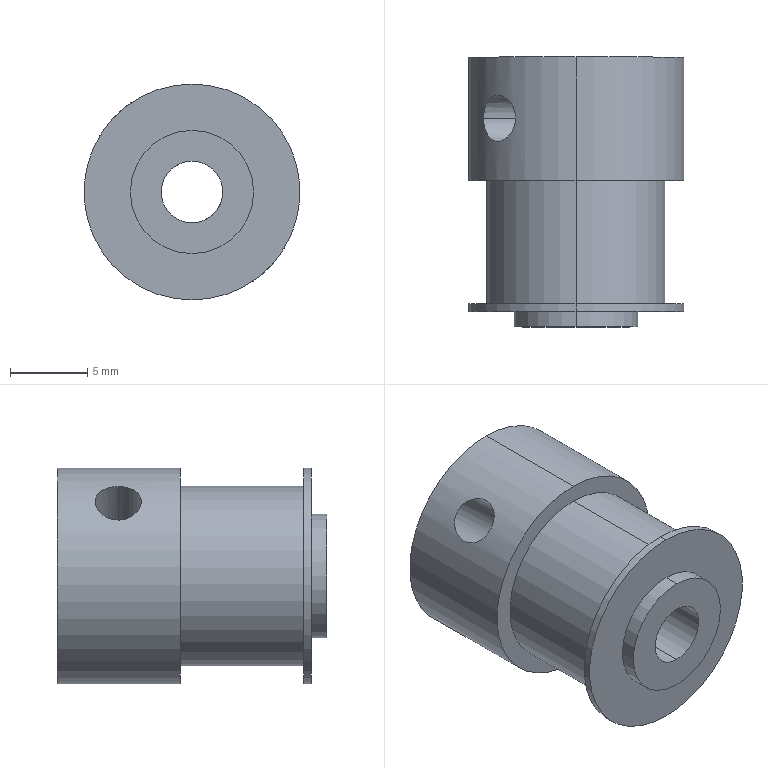Part | SolidWorks | features BaseBody 1 | 1 solid | 19 faces | box 14 x 17.5 x 14 mm | volume 1918 mm3 | cylinder 14 | plane 5 | commonest cylinder face diameters 3 x4 14 x4 4 x2 8 x2 11.64 x2
STEP:
#1=CARTESIAN_POINT('',(-3.92,13.536,5.799));
#2=VERTEX_POINT('',#1);
#3=CARTESIAN_POINT('',(-5.988,13.536,3.626));
#4=VERTEX_POINT('',#3);
#5=CARTESIAN_POINT('',(-3.92,13.536,5.799));
#6=CARTESIAN_POINT('',(-3.92,13.34,5.799));
#7=CARTESIAN_POINT('',(-3.954,13.142,5.777));
#8=CARTESIAN_POINT('',(-4.079,12.781,5.689));
#9=CARTESIAN_POINT('',(-4.171,12.615,5.623));
#10=CARTESIAN_POINT('',(-4.337,12.407,5.495));
#11=CARTESIAN_POINT('',(-4.398,12.344,5.446));
#12=CARTESIAN_POINT('',(-4.524,12.235,5.342));
#13=CARTESIAN_POINT('',(-4.59,12.189,5.286));
#14=CARTESIAN_POINT('',(-4.794,12.076,5.104));
#15=CARTESIAN_POINT('',(-4.935,12.036,4.968));
#16=CARTESIAN_POINT('',(-5.14,12.036,4.753));
#17=CARTESIAN_POINT('',(-5.205,12.046,4.681));
#18=CARTESIAN_POINT('',(-5.332,12.084,4.536));
#19=CARTESIAN_POINT('',(-5.394,12.113,4.463));
#20=CARTESIAN_POINT('',(-5.565,12.226,4.25));
#21=CARTESIAN_POINT('',(-5.664,12.337,4.115));
#22=CARTESIAN_POINT('',(-5.824,12.613,3.886));
#23=CARTESIAN_POINT('',(-5.885,12.779,3.791));
#24=CARTESIAN_POINT('',(-5.967,13.14,3.661));
#25=CARTESIAN_POINT('',(-5.988,13.337,3.626));
#26=CARTESIAN_POINT('',(-5.988,13.536,3.626));
#27=B_SPLINE_CURVE_WITH_KNOTS('',3,(#5,#6,#7,#8,#9,#10,#11,#12,#13,#14,#15,#16,#17,#18,#19,#20,#21,#22,#23,#24,#25,#26),.UNSPECIFIED.,.F.,.F.,(4,2,2,2,2,2,2,2,2,2,4),(0.004703,0.005291,0.005879,0.006173,0.006467,0.007054,0.007348,0.007642,0.00823,0.008818,0.009405),.UNSPECIFIED.);
#28=EDGE_CURVE('',#2,#4,#27,.T.);
#29=ORIENTED_EDGE('',*,*,#28,.F.);
#30=CARTESIAN_POINT('',(0.07529,13.536,1.999));
#31=VERTEX_POINT('',#30);
#32=CARTESIAN_POINT('',(6.106,13.536,-3.738));
#33=DIRECTION('',(0.7246,0.,-0.6892));
#34=VECTOR('',#33,1000.);
#35=LINE('',#32,#34);
#36=EDGE_CURVE('',#2,#31,#35,.T.);
#37=ORIENTED_EDGE('',*,*,#36,.T.);
#38=CARTESIAN_POINT('',(0.,13.149,2.));
#39=VERTEX_POINT('',#38);
#40=CARTESIAN_POINT('',(0.07529,13.536,1.999));
#41=CARTESIAN_POINT('',(0.07529,13.47,1.999));
#42=CARTESIAN_POINT('',(0.06851,13.404,1.999));
#43=CARTESIAN_POINT('',(0.04292,13.274,2.));
#44=CARTESIAN_POINT('',(0.02403,13.211,2.));
#45=CARTESIAN_POINT('',(0.,13.149,2.));
#46=B_SPLINE_CURVE_WITH_KNOTS('',3,(#40,#41,#42,#43,#44,#45),.UNSPECIFIED.,.F.,.F.,(4,2,4),(0.004899,0.005095,0.005291),.UNSPECIFIED.);
#47=EDGE_CURVE('',#31,#39,#46,.T.);
#48=ORIENTED_EDGE('',*,*,#47,.T.);
#49=CARTESIAN_POINT('',(-1.992,13.536,-0.1751));
#50=VERTEX_POINT('',#49);
#51=CARTESIAN_POINT('',(0.,13.149,2.));
#52=CARTESIAN_POINT('',(-0.06898,12.971,2.));
#53=CARTESIAN_POINT('',(-0.1759,12.813,1.996));
#54=CARTESIAN_POINT('',(-0.4253,12.53,1.958));
#55=CARTESIAN_POINT('',(-0.569,12.406,1.924));
#56=CARTESIAN_POINT('',(-0.7916,12.256,1.838));
#57=CARTESIAN_POINT('',(-0.8669,12.212,1.804));
#58=CARTESIAN_POINT('',(-1.019,12.136,1.723));
#59=CARTESIAN_POINT('',(-1.096,12.105,1.675));
#60=CARTESIAN_POINT('',(-1.32,12.036,1.514));
#61=CARTESIAN_POINT('',(-1.46,12.025,1.379));
#62=CARTESIAN_POINT('',(-1.633,12.061,1.158));
#63=CARTESIAN_POINT('',(-1.686,12.082,1.08));
#64=CARTESIAN_POINT('',(-1.776,12.14,0.9237));
#65=CARTESIAN_POINT('',(-1.815,12.176,0.8447));
#66=CARTESIAN_POINT('',(-1.913,12.306,0.6092));
#67=CARTESIAN_POINT('',(-1.952,12.417,0.4576));
#68=CARTESIAN_POINT('',(-1.996,12.677,0.1855));
#69=CARTESIAN_POINT('',(-2.001,12.826,0.06354));
#70=CARTESIAN_POINT('',(-1.999,13.158,-0.1174));
#71=CARTESIAN_POINT('',(-1.992,13.345,-0.1751));
#72=CARTESIAN_POINT('',(-1.992,13.536,-0.1751));
#73=B_SPLINE_CURVE_WITH_KNOTS('',3,(#51,#52,#53,#54,#55,#56,#57,#58,#59,#60,#61,#62,#63,#64,#65,#66,#67,#68,#69,#70,#71,#72),.UNSPECIFIED.,.F.,.F.,(4,2,2,2,2,2,2,2,2,2,4),(0.005291,0.005853,0.006416,0.006697,0.006978,0.00754,0.007821,0.008102,0.008665,0.009227,0.009789),.UNSPECIFIED.);
#74=EDGE_CURVE('',#39,#50,#73,.T.);
#75=ORIENTED_EDGE('',*,*,#74,.T.);
#76=CARTESIAN_POINT('',(4.038,13.536,-5.911));
#77=DIRECTION('',(0.7246,0.,-0.6892));
#78=VECTOR('',#77,1000.);
#79=LINE('',#76,#78);
#80=EDGE_CURVE('',#4,#50,#79,.T.);
#81=ORIENTED_EDGE('',*,*,#80,.F.);
#82=EDGE_LOOP('',(#29,#37,#48,#75,#81));
#83=FACE_OUTER_BOUND('',#82,.T.);
#84=CARTESIAN_POINT('',(5.072,13.536,-4.824));
#85=DIRECTION('',(0.7246,0.,-0.6892));
#86=DIRECTION('',(-0.6892,0.,-0.7246));
#87=AXIS2_PLACEMENT_3D('',#84,#85,#86);
#88=CYLINDRICAL_SURFACE('',#87,1.5);
#89=ADVANCED_FACE('',(#83),#88,.F.);
#90=CARTESIAN_POINT('',(0.,13.149,-2.));
#91=VERTEX_POINT('',#90);
#92=CARTESIAN_POINT('',(1.992,13.536,0.1751));
#93=VERTEX_POINT('',#92);
#94=CARTESIAN_POINT('',(0.,13.149,-2.));
#95=CARTESIAN_POINT('',(0.06867,12.972,-2.));
#96=CARTESIAN_POINT('',(0.1764,12.812,-1.996));
#97=CARTESIAN_POINT('',(0.4248,12.531,-1.958));
#98=CARTESIAN_POINT('',(0.5678,12.407,-1.924));
#99=CARTESIAN_POINT('',(0.7916,12.256,-1.838));
#100=CARTESIAN_POINT('',(0.8673,12.212,-1.804));
#101=CARTESIAN_POINT('',(1.02,12.136,-1.722));
#102=CARTESIAN_POINT('',(1.098,12.104,-1.674));
#103=CARTESIAN_POINT('',(1.246,12.059,-1.567));
#104=CARTESIAN_POINT('',(1.319,12.044,-1.506));
#105=CARTESIAN_POINT('',(1.456,12.033,-1.375));
#106=CARTESIAN_POINT('',(1.519,12.037,-1.305));
#107=CARTESIAN_POINT('',(1.692,12.073,-1.083));
#108=CARTESIAN_POINT('',(1.783,12.134,-0.9215));
#109=CARTESIAN_POINT('',(1.913,12.306,-0.6088));
#110=CARTESIAN_POINT('',(1.952,12.418,-0.4567));
#111=CARTESIAN_POINT('',(1.996,12.677,-0.1853));
#112=CARTESIAN_POINT('',(2.001,12.827,-0.063));
#113=CARTESIAN_POINT('',(1.999,13.158,0.1174));
#114=CARTESIAN_POINT('',(1.992,13.344,0.1751));
#115=CARTESIAN_POINT('',(1.992,13.536,0.1751));
#116=B_SPLINE_CURVE_WITH_KNOTS('',3,(#94,#95,#96,#97,#98,#99,#100,#101,#102,#103,#104,#105,#106,#107,#108,#109,#110,#111,#112,#113,#114,#115),.UNSPECIFIED.,.F.,.F.,(4,2,2,2,2,2,2,2,2,2,4),(0.0007898,0.001356,0.001923,0.002206,0.00249,0.002773,0.003056,0.003623,0.004189,0.004756,0.005323),.UNSPECIFIED.);
#117=EDGE_CURVE('',#91,#93,#116,.T.);
#118=ORIENTED_EDGE('',*,*,#117,.T.);
#119=CARTESIAN_POINT('',(5.988,13.536,-3.626));
#120=VERTEX_POINT('',#119);
#121=CARTESIAN_POINT('',(6.106,13.536,-3.738));
#122=DIRECTION('',(0.7246,0.,-0.6892));
#123=VECTOR('',#122,1000.);
#124=LINE('',#121,#123);
#125=EDGE_CURVE('',#93,#120,#124,.T.);
#126=ORIENTED_EDGE('',*,*,#125,.T.);
#127=CARTESIAN_POINT('',(3.92,13.536,-5.799));
#128=VERTEX_POINT('',#127);
#129=CARTESIAN_POINT('',(3.92,13.536,-5.799));
#130=CARTESIAN_POINT('',(3.92,13.437,-5.799));
#131=CARTESIAN_POINT('',(3.929,13.339,-5.794));
#132=CARTESIAN_POINT('',(3.961,13.147,-5.772));
#133=CARTESIAN_POINT('',(3.985,13.052,-5.755));
#134=CARTESIAN_POINT('',(4.048,12.87,-5.711));
#135=CARTESIAN_POINT('',(4.087,12.784,-5.683));
#136=CARTESIAN_POINT('',(4.176,12.621,-5.618));
#137=CARTESIAN_POINT('',(4.227,12.544,-5.58));
#138=CARTESIAN_POINT('',(4.393,12.337,-5.452));
#139=CARTESIAN_POINT('',(4.523,12.226,-5.345));
#140=CARTESIAN_POINT('',(4.794,12.076,-5.104));
#141=CARTESIAN_POINT('',(4.936,12.036,-4.967));
#142=CARTESIAN_POINT('',(5.139,12.036,-4.754));
#143=CARTESIAN_POINT('',(5.206,12.046,-4.68));
#144=CARTESIAN_POINT('',(5.333,12.085,-4.535));
#145=CARTESIAN_POINT('',(5.394,12.113,-4.463));
#146=CARTESIAN_POINT('',(5.565,12.226,-4.25));
#147=CARTESIAN_POINT('',(5.664,12.336,-4.116));
#148=CARTESIAN_POINT('',(5.785,12.545,-3.942));
#149=CARTESIAN_POINT('',(5.82,12.621,-3.89));
#150=CARTESIAN_POINT('',(5.88,12.783,-3.798));
#151=CARTESIAN_POINT('',(5.906,12.871,-3.758));
#152=CARTESIAN_POINT('',(5.947,13.052,-3.693));
#153=CARTESIAN_POINT('',(5.962,13.146,-3.668));
#154=CARTESIAN_POINT('',(5.983,13.339,-3.634));
#155=CARTESIAN_POINT('',(5.988,13.438,-3.626));
#156=CARTESIAN_POINT('',(5.988,13.536,-3.626));
#157=B_SPLINE_CURVE_WITH_KNOTS('',3,(#129,#130,#131,#132,#133,#134,#135,#136,#137,#138,#139,#140,#141,#142,#143,#144,#145,#146,#147,#148,#149,#150,#151,#152,#153,#154,#155,#156),.UNSPECIFIED.,.F.,.F.,(4,2,2,2,2,2,2,2,2,2,2,2,2,4),(0.,0.000294,0.0005879,0.0008819,0.001176,0.001764,0.002352,0.002646,0.00294,0.003527,0.003821,0.004115,0.004409,0.004703),.UNSPECIFIED.);
#158=EDGE_CURVE('',#128,#120,#157,.T.);
#159=ORIENTED_EDGE('',*,*,#158,.F.);
#160=CARTESIAN_POINT('',(-0.07529,13.536,-1.999));
#161=VERTEX_POINT('',#160);
#162=CARTESIAN_POINT('',(4.038,13.536,-5.911));
#163=DIRECTION('',(0.7246,0.,-0.6892));
#164=VECTOR('',#163,1000.);
#165=LINE('',#162,#164);
#166=EDGE_CURVE('',#161,#128,#165,.T.);
#167=ORIENTED_EDGE('',*,*,#166,.F.);
#168=CARTESIAN_POINT('',(-0.07529,13.536,-1.999));
#169=CARTESIAN_POINT('',(-0.07529,13.47,-1.999));
#170=CARTESIAN_POINT('',(-0.06861,13.404,-1.999));
#171=CARTESIAN_POINT('',(-0.04307,13.275,-2.));
#172=CARTESIAN_POINT('',(-0.02394,13.211,-2.));
#173=CARTESIAN_POINT('',(0.,13.149,-2.));
#174=B_SPLINE_CURVE_WITH_KNOTS('',3,(#168,#169,#170,#171,#172,#173),.UNSPECIFIED.,.F.,.F.,(4,2,4),(0.0003947,0.0005923,0.0007898),.UNSPECIFIED.);
#175=EDGE_CURVE('',#161,#91,#174,.T.);
#176=ORIENTED_EDGE('',*,*,#175,.T.);
#177=EDGE_LOOP('',(#118,#126,#159,#167,#176));
#178=FACE_OUTER_BOUND('',#177,.T.);
#179=CARTESIAN_POINT('',(5.072,13.536,-4.824));
#180=DIRECTION('',(0.7246,0.,-0.6892));
#181=DIRECTION('',(-0.6892,0.,-0.7246));
#182=AXIS2_PLACEMENT_3D('',#179,#180,#181);
#183=CYLINDRICAL_SURFACE('',#182,1.5);
#184=ADVANCED_FACE('',(#178),#183,.F.);
#185=ORIENTED_EDGE('',*,*,#158,.T.);
#186=CARTESIAN_POINT('',(5.988,13.536,-3.626));
#187=CARTESIAN_POINT('',(5.988,13.732,-3.626));
#188=CARTESIAN_POINT('',(5.967,13.93,-3.66));
#189=CARTESIAN_POINT('',(5.886,14.291,-3.79));
#190=CARTESIAN_POINT('',(5.825,14.458,-3.885));
#191=CARTESIAN_POINT('',(5.705,14.665,-4.057));
#192=CARTESIAN_POINT('',(5.66,14.729,-4.12));
#193=CARTESIAN_POINT('',(5.562,14.837,-4.251));
#194=CARTESIAN_POINT('',(5.509,14.883,-4.32));
#195=CARTESIAN_POINT('',(5.337,14.997,-4.533));
#196=CARTESIAN_POINT('',(5.209,15.036,-4.68));
#197=CARTESIAN_POINT('',(5.004,15.036,-4.896));
#198=CARTESIAN_POINT('',(4.935,15.027,-4.965));
#199=CARTESIAN_POINT('',(4.797,14.988,-5.099));
#200=CARTESIAN_POINT('',(4.727,14.959,-5.164));
#201=CARTESIAN_POINT('',(4.523,14.847,-5.345));
#202=CARTESIAN_POINT('',(4.393,14.735,-5.452));
#203=CARTESIAN_POINT('',(4.173,14.46,-5.622));
#204=CARTESIAN_POINT('',(4.08,14.293,-5.689));
#205=CARTESIAN_POINT('',(3.955,13.932,-5.776));
#206=CARTESIAN_POINT('',(3.92,13.735,-5.799));
#207=CARTESIAN_POINT('',(3.92,13.536,-5.799));
#208=B_SPLINE_CURVE_WITH_KNOTS('',3,(#186,#187,#188,#189,#190,#191,#192,#193,#194,#195,#196,#197,#198,#199,#200,#201,#202,#203,#204,#205,#206,#207),.UNSPECIFIED.,.F.,.F.,(4,2,2,2,2,2,2,2,2,2,4),(0.004703,0.005291,0.005879,0.006173,0.006467,0.007054,0.007348,0.007642,0.00823,0.008818,0.009405),.UNSPECIFIED.);
#209=EDGE_CURVE('',#120,#128,#208,.T.);
#210=ORIENTED_EDGE('',*,*,#209,.T.);
#211=EDGE_LOOP('',(#185,#210));
#212=FACE_BOUND('',#211,.T.);
#213=CARTESIAN_POINT('',(0.,17.5,7.));
#214=VERTEX_POINT('',#213);
#215=CARTESIAN_POINT('',(0.,17.5,-7.));
#216=VERTEX_POINT('',#215);
#217=CARTESIAN_POINT('',(0.,17.5,0.));
#218=DIRECTION('',(0.,1.,0.));
#219=DIRECTION('',(0.,0.,1.));
#220=AXIS2_PLACEMENT_3D('',#217,#218,#219);
#221=CIRCLE('',#220,7.);
#222=EDGE_CURVE('',#214,#216,#221,.T.);
#223=ORIENTED_EDGE('',*,*,#222,.F.);
#224=CARTESIAN_POINT('',(0.,9.5,7.));
#225=VERTEX_POINT('',#224);
#226=CARTESIAN_POINT('',(0.,17.5,7.));
#227=DIRECTION('',(0.,-1.,0.));
#228=VECTOR('',#227,1000.);
#229=LINE('',#226,#228);
#230=EDGE_CURVE('',#214,#225,#229,.T.);
#231=ORIENTED_EDGE('',*,*,#230,.T.);
#232=CARTESIAN_POINT('',(0.,9.5,-7.));
#233=VERTEX_POINT('',#232);
#234=CARTESIAN_POINT('',(0.,9.5,0.));
#235=DIRECTION('',(0.,1.,0.));
#236=DIRECTION('',(0.,0.,1.));
#237=AXIS2_PLACEMENT_3D('',#234,#235,#236);
#238=CIRCLE('',#237,7.);
#239=EDGE_CURVE('',#225,#233,#238,.T.);
#240=ORIENTED_EDGE('',*,*,#239,.T.);
#241=CARTESIAN_POINT('',(0.,17.5,-7.));
#242=DIRECTION('',(0.,-1.,0.));
#243=VECTOR('',#242,1000.);
#244=LINE('',#241,#243);
#245=EDGE_CURVE('',#216,#233,#244,.T.);
#246=ORIENTED_EDGE('',*,*,#245,.F.);
#247=EDGE_LOOP('',(#223,#231,#240,#246));
#248=FACE_OUTER_BOUND('',#247,.T.);
#249=CARTESIAN_POINT('',(0.,17.5,0.));
#250=DIRECTION('',(0.,-1.,0.));
#251=DIRECTION('',(0.,0.,-1.));
#252=AXIS2_PLACEMENT_3D('',#249,#250,#251);
#253=CYLINDRICAL_SURFACE('',#252,7.);
#254=ADVANCED_FACE('',(#212,#248),#253,.T.);
#255=CARTESIAN_POINT('',(0.,9.5,5.82));
#256=VERTEX_POINT('',#255);
#257=CARTESIAN_POINT('',(0.,9.5,-5.82));
#258=VERTEX_POINT('',#257);
#259=CARTESIAN_POINT('',(0.,9.5,0.));
#260=DIRECTION('',(0.,1.,0.));
#261=DIRECTION('',(0.,0.,1.));
#262=AXIS2_PLACEMENT_3D('',#259,#260,#261);
#263=CIRCLE('',#262,5.82);
#264=EDGE_CURVE('',#256,#258,#263,.T.);
#265=ORIENTED_EDGE('',*,*,#264,.F.);
#266=CARTESIAN_POINT('',(0.,1.5,5.82));
#267=VERTEX_POINT('',#266);
#268=CARTESIAN_POINT('',(0.,9.5,5.82));
#269=DIRECTION('',(0.,-1.,0.));
#270=VECTOR('',#269,1000.);
#271=LINE('',#268,#270);
#272=EDGE_CURVE('',#256,#267,#271,.T.);
#273=ORIENTED_EDGE('',*,*,#272,.T.);
#274=CARTESIAN_POINT('',(0.,1.5,-5.82));
#275=VERTEX_POINT('',#274);
#276=CARTESIAN_POINT('',(0.,1.5,0.));
#277=DIRECTION('',(0.,1.,0.));
#278=DIRECTION('',(0.,0.,1.));
#279=AXIS2_PLACEMENT_3D('',#276,#277,#278);
#280=CIRCLE('',#279,5.82);
#281=EDGE_CURVE('',#267,#275,#280,.T.);
#282=ORIENTED_EDGE('',*,*,#281,.T.);
#283=CARTESIAN_POINT('',(0.,9.5,-5.82));
#284=DIRECTION('',(0.,-1.,0.));
#285=VECTOR('',#284,1000.);
#286=LINE('',#283,#285);
#287=EDGE_CURVE('',#258,#275,#286,.T.);
#288=ORIENTED_EDGE('',*,*,#287,.F.);
#289=EDGE_LOOP('',(#265,#273,#282,#288));
#290=FACE_OUTER_BOUND('',#289,.T.);
#291=CARTESIAN_POINT('',(0.,9.5,0.));
#292=DIRECTION('',(0.,-1.,0.));
#293=DIRECTION('',(0.,0.,-1.));
#294=AXIS2_PLACEMENT_3D('',#291,#292,#293);
#295=CYLINDRICAL_SURFACE('',#294,5.82);
#296=ADVANCED_FACE('',(#290),#295,.T.);
#297=CARTESIAN_POINT('',(0.,1.5,7.));
#298=VERTEX_POINT('',#297);
#299=CARTESIAN_POINT('',(0.,1.5,-7.));
#300=VERTEX_POINT('',#299);
#301=CARTESIAN_POINT('',(0.,1.5,0.));
#302=DIRECTION('',(0.,1.,0.));
#303=DIRECTION('',(0.,0.,1.));
#304=AXIS2_PLACEMENT_3D('',#301,#302,#303);
#305=CIRCLE('',#304,7.);
#306=EDGE_CURVE('',#298,#300,#305,.T.);
#307=ORIENTED_EDGE('',*,*,#306,.F.);
#308=CARTESIAN_POINT('',(0.,1.,7.));
#309=VERTEX_POINT('',#308);
#310=CARTESIAN_POINT('',(0.,1.5,7.));
#311=DIRECTION('',(0.,-1.,0.));
#312=VECTOR('',#311,1000.);
#313=LINE('',#310,#312);
#314=EDGE_CURVE('',#298,#309,#313,.T.);
#315=ORIENTED_EDGE('',*,*,#314,.T.);
#316=CARTESIAN_POINT('',(0.,1.,-7.));
#317=VERTEX_POINT('',#316);
#318=CARTESIAN_POINT('',(0.,1.,0.));
#319=DIRECTION('',(0.,1.,0.));
#320=DIRECTION('',(0.,0.,1.));
#321=AXIS2_PLACEMENT_3D('',#318,#319,#320);
#322=CIRCLE('',#321,7.);
#323=EDGE_CURVE('',#309,#317,#322,.T.);
#324=ORIENTED_EDGE('',*,*,#323,.T.);
#325=CARTESIAN_POINT('',(0.,1.5,-7.));
#326=DIRECTION('',(0.,-1.,0.));
#327=VECTOR('',#326,1000.);
#328=LINE('',#325,#327);
#329=EDGE_CURVE('',#300,#317,#328,.T.);
#330=ORIENTED_EDGE('',*,*,#329,.F.);
#331=EDGE_LOOP('',(#307,#315,#324,#330));
#332=FACE_OUTER_BOUND('',#331,.T.);
#333=CARTESIAN_POINT('',(0.,1.5,0.));
#334=DIRECTION('',(0.,-1.,0.));
#335=DIRECTION('',(0.,0.,-1.));
#336=AXIS2_PLACEMENT_3D('',#333,#334,#335);
#337=CYLINDRICAL_SURFACE('',#336,7.);
#338=ADVANCED_FACE('',(#332),#337,.T.);
#339=CARTESIAN_POINT('',(0.,17.5,-2.));
#340=VERTEX_POINT('',#339);
#341=CARTESIAN_POINT('',(0.,17.5,2.));
#342=VERTEX_POINT('',#341);
#343=CARTESIAN_POINT('',(0.,17.5,0.));
#344=DIRECTION('',(0.,1.,0.));
#345=DIRECTION('',(0.,0.,1.));
#346=AXIS2_PLACEMENT_3D('',#343,#344,#345);
#347=CIRCLE('',#346,2.);
#348=EDGE_CURVE('',#340,#342,#347,.T.);
#349=ORIENTED_EDGE('',*,*,#348,.T.);
#350=CARTESIAN_POINT('',(0.,13.924,2.));
#351=VERTEX_POINT('',#350);
#352=CARTESIAN_POINT('',(0.,1.,2.));
#353=DIRECTION('',(0.,-1.,0.));
#354=VECTOR('',#353,1000.);
#355=LINE('',#352,#354);
#356=EDGE_CURVE('',#342,#351,#355,.T.);
#357=ORIENTED_EDGE('',*,*,#356,.T.);
#358=CARTESIAN_POINT('',(-1.992,13.536,-0.1751));
#359=CARTESIAN_POINT('',(-1.992,13.632,-0.1751));
#360=CARTESIAN_POINT('',(-1.994,13.725,-0.1613));
#361=CARTESIAN_POINT('',(-1.997,13.906,-0.1106));
#362=CARTESIAN_POINT('',(-1.999,13.995,-0.07313));
#363=CARTESIAN_POINT('',(-2.001,14.245,0.06217));
#364=CARTESIAN_POINT('',(-1.996,14.394,0.1841));
#365=CARTESIAN_POINT('',(-1.952,14.654,0.4554));
#366=CARTESIAN_POINT('',(-1.913,14.765,0.6074));
#367=CARTESIAN_POINT('',(-1.786,14.936,0.9159));
#368=CARTESIAN_POINT('',(-1.695,14.997,1.077));
#369=CARTESIAN_POINT('',(-1.465,15.048,1.374));
#370=CARTESIAN_POINT('',(-1.325,15.037,1.509));
#371=CARTESIAN_POINT('',(-1.026,14.947,1.727));
#372=CARTESIAN_POINT('',(-0.8688,14.868,1.809));
#373=CARTESIAN_POINT('',(-0.5697,14.667,1.924));
#374=CARTESIAN_POINT('',(-0.4258,14.543,1.958));
#375=CARTESIAN_POINT('',(-0.1768,14.261,1.996));
#376=CARTESIAN_POINT('',(-0.06869,14.101,2.));
#377=CARTESIAN_POINT('',(0.,13.924,2.));
#378=B_SPLINE_CURVE_WITH_KNOTS('',3,(#358,#359,#360,#361,#362,#363,#364,#365,#366,#367,#368,#369,#370,#371,#372,#373,#374,#375,#376,#377),.UNSPECIFIED.,.F.,.F.,(4,2,2,2,2,2,2,2,2,4),(0.,0.0002817,0.0005634,0.001127,0.00169,0.002254,0.002817,0.003381,0.003944,0.004507),.UNSPECIFIED.);
#379=EDGE_CURVE('',#50,#351,#378,.T.);
#380=ORIENTED_EDGE('',*,*,#379,.F.);
#381=ORIENTED_EDGE('',*,*,#74,.F.);
#382=CARTESIAN_POINT('',(0.,0.,2.));
#383=VERTEX_POINT('',#382);
#384=CARTESIAN_POINT('',(0.,1.,2.));
#385=DIRECTION('',(0.,-1.,0.));
#386=VECTOR('',#385,1000.);
#387=LINE('',#384,#386);
#388=EDGE_CURVE('',#39,#383,#387,.T.);
#389=ORIENTED_EDGE('',*,*,#388,.T.);
#390=CARTESIAN_POINT('',(0.,0.,-2.));
#391=VERTEX_POINT('',#390);
#392=CARTESIAN_POINT('',(0.,0.,0.));
#393=DIRECTION('',(0.,1.,0.));
#394=DIRECTION('',(0.,0.,1.));
#395=AXIS2_PLACEMENT_3D('',#392,#393,#394);
#396=CIRCLE('',#395,2.);
#397=EDGE_CURVE('',#391,#383,#396,.T.);
#398=ORIENTED_EDGE('',*,*,#397,.F.);
#399=CARTESIAN_POINT('',(0.,1.,-2.));
#400=DIRECTION('',(0.,-1.,0.));
#401=VECTOR('',#400,1000.);
#402=LINE('',#399,#401);
#403=EDGE_CURVE('',#91,#391,#402,.T.);
#404=ORIENTED_EDGE('',*,*,#403,.F.);
#405=ORIENTED_EDGE('',*,*,#175,.F.);
#406=CARTESIAN_POINT('',(0.,13.924,-2.));
#407=VERTEX_POINT('',#406);
#408=CARTESIAN_POINT('',(0.,13.924,-2.));
#409=CARTESIAN_POINT('',(-0.0241,13.861,-2.));
#410=CARTESIAN_POINT('',(-0.04289,13.798,-2.));
#411=CARTESIAN_POINT('',(-0.0685,13.669,-1.999));
#412=CARTESIAN_POINT('',(-0.07529,13.603,-1.999));
#413=CARTESIAN_POINT('',(-0.07529,13.536,-1.999));
#414=B_SPLINE_CURVE_WITH_KNOTS('',3,(#408,#409,#410,#411,#412,#413),.UNSPECIFIED.,.F.,.F.,(4,2,4),(0.,0.0001974,0.0003947),.UNSPECIFIED.);
#415=EDGE_CURVE('',#407,#161,#414,.T.);
#416=ORIENTED_EDGE('',*,*,#415,.F.);
#417=CARTESIAN_POINT('',(0.,1.,-2.));
#418=DIRECTION('',(0.,-1.,0.));
#419=VECTOR('',#418,1000.);
#420=LINE('',#417,#419);
#421=EDGE_CURVE('',#340,#407,#420,.T.);
#422=ORIENTED_EDGE('',*,*,#421,.F.);
#423=EDGE_LOOP('',(#349,#357,#380,#381,#389,#398,#404,#405,#416,#422));
#424=FACE_OUTER_BOUND('',#423,.T.);
#425=CARTESIAN_POINT('',(0.,1.,0.));
#426=DIRECTION('',(0.,-1.,0.));
#427=DIRECTION('',(0.,0.,-1.));
#428=AXIS2_PLACEMENT_3D('',#425,#426,#427);
#429=CYLINDRICAL_SURFACE('',#428,2.);
#430=ADVANCED_FACE('',(#424),#429,.F.);
#431=CARTESIAN_POINT('',(0.,1.,4.));
#432=VERTEX_POINT('',#431);
#433=CARTESIAN_POINT('',(0.,1.,-4.));
#434=VERTEX_POINT('',#433);
#435=CARTESIAN_POINT('',(0.,1.,0.));
#436=DIRECTION('',(0.,1.,0.));
#437=DIRECTION('',(0.,0.,1.));
#438=AXIS2_PLACEMENT_3D('',#435,#436,#437);
#439=CIRCLE('',#438,4.);
#440=EDGE_CURVE('',#432,#434,#439,.T.);
#441=ORIENTED_EDGE('',*,*,#440,.F.);
#442=CARTESIAN_POINT('',(0.,0.,4.));
#443=VERTEX_POINT('',#442);
#444=CARTESIAN_POINT('',(0.,1.,4.));
#445=DIRECTION('',(0.,-1.,0.));
#446=VECTOR('',#445,1000.);
#447=LINE('',#444,#446);
#448=EDGE_CURVE('',#432,#443,#447,.T.);
#449=ORIENTED_EDGE('',*,*,#448,.T.);
#450=CARTESIAN_POINT('',(0.,0.,-4.));
#451=VERTEX_POINT('',#450);
#452=CARTESIAN_POINT('',(0.,0.,0.));
#453=DIRECTION('',(0.,1.,0.));
#454=DIRECTION('',(0.,0.,1.));
#455=AXIS2_PLACEMENT_3D('',#452,#453,#454);
#456=CIRCLE('',#455,4.);
#457=EDGE_CURVE('',#443,#451,#456,.T.);
#458=ORIENTED_EDGE('',*,*,#457,.T.);
#459=CARTESIAN_POINT('',(0.,1.,-4.));
#460=DIRECTION('',(0.,-1.,0.));
#461=VECTOR('',#460,1000.);
#462=LINE('',#459,#461);
#463=EDGE_CURVE('',#434,#451,#462,.T.);
#464=ORIENTED_EDGE('',*,*,#463,.F.);
#465=EDGE_LOOP('',(#441,#449,#458,#464));
#466=FACE_OUTER_BOUND('',#465,.T.);
#467=CARTESIAN_POINT('',(0.,1.,0.));
#468=DIRECTION('',(0.,-1.,0.));
#469=DIRECTION('',(0.,0.,-1.));
#470=AXIS2_PLACEMENT_3D('',#467,#468,#469);
#471=CYLINDRICAL_SURFACE('',#470,4.);
#472=ADVANCED_FACE('',(#466),#471,.T.);
#473=CARTESIAN_POINT('',(0.,1.5,0.));
#474=DIRECTION('',(0.,1.,0.));
#475=DIRECTION('',(0.,0.,1.));
#476=AXIS2_PLACEMENT_3D('',#473,#474,#475);
#477=CIRCLE('',#476,7.);
#478=EDGE_CURVE('',#300,#298,#477,.T.);
#479=ORIENTED_EDGE('',*,*,#478,.T.);
#480=ORIENTED_EDGE('',*,*,#306,.T.);
#481=EDGE_LOOP('',(#479,#480));
#482=FACE_OUTER_BOUND('',#481,.T.);
#483=CARTESIAN_POINT('',(0.,1.5,0.));
#484=DIRECTION('',(0.,1.,0.));
#485=DIRECTION('',(0.,0.,1.));
#486=AXIS2_PLACEMENT_3D('',#483,#484,#485);
#487=CIRCLE('',#486,5.82);
#488=EDGE_CURVE('',#275,#267,#487,.T.);
#489=ORIENTED_EDGE('',*,*,#488,.F.);
#490=ORIENTED_EDGE('',*,*,#281,.F.);
#491=EDGE_LOOP('',(#489,#490));
#492=FACE_BOUND('',#491,.T.);
#493=CARTESIAN_POINT('',(0.,1.5,0.));
#494=DIRECTION('',(0.,1.,0.));
#495=DIRECTION('',(0.,0.,1.));
#496=AXIS2_PLACEMENT_3D('',#493,#494,#495);
#497=PLANE('',#496);
#498=ADVANCED_FACE('',(#482,#492),#497,.T.);
#499=CARTESIAN_POINT('',(0.,0.,0.));
#500=DIRECTION('',(0.,1.,0.));
#501=DIRECTION('',(0.,0.,1.));
#502=AXIS2_PLACEMENT_3D('',#499,#500,#501);
#503=CIRCLE('',#502,4.);
#504=EDGE_CURVE('',#451,#443,#503,.T.);
#505=ORIENTED_EDGE('',*,*,#504,.F.);
#506=ORIENTED_EDGE('',*,*,#457,.F.);
#507=EDGE_LOOP('',(#505,#506));
#508=FACE_OUTER_BOUND('',#507,.T.);
#509=ORIENTED_EDGE('',*,*,#397,.T.);
#510=CARTESIAN_POINT('',(0.,0.,0.));
#511=DIRECTION('',(0.,1.,0.));
#512=DIRECTION('',(0.,0.,1.));
#513=AXIS2_PLACEMENT_3D('',#510,#511,#512);
#514=CIRCLE('',#513,2.);
#515=EDGE_CURVE('',#383,#391,#514,.T.);
#516=ORIENTED_EDGE('',*,*,#515,.T.);
#517=EDGE_LOOP('',(#509,#516));
#518=FACE_BOUND('',#517,.T.);
#519=CARTESIAN_POINT('',(0.,0.,0.));
#520=DIRECTION('',(0.,1.,0.));
#521=DIRECTION('',(0.,0.,1.));
#522=AXIS2_PLACEMENT_3D('',#519,#520,#521);
#523=PLANE('',#522);
#524=ADVANCED_FACE('',(#508,#518),#523,.F.);
#525=ORIENTED_EDGE('',*,*,#448,.F.);
#526=CARTESIAN_POINT('',(0.,1.,0.));
#527=DIRECTION('',(0.,1.,0.));
#528=DIRECTION('',(0.,0.,1.));
#529=AXIS2_PLACEMENT_3D('',#526,#527,#528);
#530=CIRCLE('',#529,4.);
#531=EDGE_CURVE('',#434,#432,#530,.T.);
#532=ORIENTED_EDGE('',*,*,#531,.F.);
#533=ORIENTED_EDGE('',*,*,#463,.T.);
#534=ORIENTED_EDGE('',*,*,#504,.T.);
#535=EDGE_LOOP('',(#525,#532,#533,#534));
#536=FACE_OUTER_BOUND('',#535,.T.);
#537=CARTESIAN_POINT('',(0.,1.,0.));
#538=DIRECTION('',(0.,-1.,0.));
#539=DIRECTION('',(0.,0.,-1.));
#540=AXIS2_PLACEMENT_3D('',#537,#538,#539);
#541=CYLINDRICAL_SURFACE('',#540,4.);
#542=ADVANCED_FACE('',(#536),#541,.T.);
#543=ORIENTED_EDGE('',*,*,#356,.F.);
#544=CARTESIAN_POINT('',(0.,17.5,0.));
#545=DIRECTION('',(0.,1.,0.));
#546=DIRECTION('',(0.,0.,1.));
#547=AXIS2_PLACEMENT_3D('',#544,#545,#546);
#548=CIRCLE('',#547,2.);
#549=EDGE_CURVE('',#342,#340,#548,.T.);
#550=ORIENTED_EDGE('',*,*,#549,.T.);
#551=ORIENTED_EDGE('',*,*,#421,.T.);
#552=CARTESIAN_POINT('',(1.992,13.536,0.1751));
#553=CARTESIAN_POINT('',(1.992,13.728,0.1751));
#554=CARTESIAN_POINT('',(1.999,13.914,0.1175));
#555=CARTESIAN_POINT('',(2.001,14.245,-0.06258));
#556=CARTESIAN_POINT('',(1.996,14.395,-0.1848));
#557=CARTESIAN_POINT('',(1.952,14.653,-0.4548));
#558=CARTESIAN_POINT('',(1.913,14.765,-0.6073));
#559=CARTESIAN_POINT('',(1.785,14.937,-0.9174));
#560=CARTESIAN_POINT('',(1.695,14.998,-1.078));
#561=CARTESIAN_POINT('',(1.464,15.048,-1.375));
#562=CARTESIAN_POINT('',(1.324,15.037,-1.51));
#563=CARTESIAN_POINT('',(1.026,14.947,-1.727));
#564=CARTESIAN_POINT('',(0.8687,14.868,-1.809));
#565=CARTESIAN_POINT('',(0.57,14.667,-1.924));
#566=CARTESIAN_POINT('',(0.4262,14.543,-1.958));
#567=CARTESIAN_POINT('',(0.1772,14.262,-1.996));
#568=CARTESIAN_POINT('',(0.06914,14.102,-2.));
#569=CARTESIAN_POINT('',(0.,13.924,-2.));
#570=B_SPLINE_CURVE_WITH_KNOTS('',3,(#552,#553,#554,#555,#556,#557,#558,#559,#560,#561,#562,#563,#564,#565,#566,#567,#568,#569),.UNSPECIFIED.,.F.,.F.,(4,2,2,2,2,2,2,2,4),(0.005323,0.005889,0.006455,0.007021,0.007587,0.008154,0.00872,0.009286,0.009852),.UNSPECIFIED.);
#571=EDGE_CURVE('',#93,#407,#570,.T.);
#572=ORIENTED_EDGE('',*,*,#571,.F.);
#573=ORIENTED_EDGE('',*,*,#117,.F.);
#574=ORIENTED_EDGE('',*,*,#403,.T.);
#575=ORIENTED_EDGE('',*,*,#515,.F.);
#576=ORIENTED_EDGE('',*,*,#388,.F.);
#577=ORIENTED_EDGE('',*,*,#47,.F.);
#578=CARTESIAN_POINT('',(0.,13.924,2.));
#579=CARTESIAN_POINT('',(0.0239,13.862,2.));
#580=CARTESIAN_POINT('',(0.04305,13.798,2.));
#581=CARTESIAN_POINT('',(0.06862,13.668,1.999));
#582=CARTESIAN_POINT('',(0.07529,13.603,1.999));
#583=CARTESIAN_POINT('',(0.07529,13.536,1.999));
#584=B_SPLINE_CURVE_WITH_KNOTS('',3,(#578,#579,#580,#581,#582,#583),.UNSPECIFIED.,.F.,.F.,(4,2,4),(0.004507,0.004703,0.004899),.UNSPECIFIED.);
#585=EDGE_CURVE('',#351,#31,#584,.T.);
#586=ORIENTED_EDGE('',*,*,#585,.F.);
#587=EDGE_LOOP('',(#543,#550,#551,#572,#573,#574,#575,#576,#577,#586));
#588=FACE_OUTER_BOUND('',#587,.T.);
#589=CARTESIAN_POINT('',(0.,1.,0.));
#590=DIRECTION('',(0.,-1.,0.));
#591=DIRECTION('',(0.,0.,-1.));
#592=AXIS2_PLACEMENT_3D('',#589,#590,#591);
#593=CYLINDRICAL_SURFACE('',#592,2.);
#594=ADVANCED_FACE('',(#588),#593,.F.);
#595=CARTESIAN_POINT('',(0.,1.,0.));
#596=DIRECTION('',(0.,1.,0.));
#597=DIRECTION('',(0.,0.,1.));
#598=AXIS2_PLACEMENT_3D('',#595,#596,#597);
#599=CIRCLE('',#598,7.);
#600=EDGE_CURVE('',#317,#309,#599,.T.);
#601=ORIENTED_EDGE('',*,*,#600,.F.);
#602=ORIENTED_EDGE('',*,*,#323,.F.);
#603=EDGE_LOOP('',(#601,#602));
#604=FACE_OUTER_BOUND('',#603,.T.);
#605=ORIENTED_EDGE('',*,*,#531,.T.);
#606=ORIENTED_EDGE('',*,*,#440,.T.);
#607=EDGE_LOOP('',(#605,#606));
#608=FACE_BOUND('',#607,.T.);
#609=CARTESIAN_POINT('',(0.,1.,0.));
#610=DIRECTION('',(0.,1.,0.));
#611=DIRECTION('',(0.,0.,1.));
#612=AXIS2_PLACEMENT_3D('',#609,#610,#611);
#613=PLANE('',#612);
#614=ADVANCED_FACE('',(#604,#608),#613,.F.);
#615=ORIENTED_EDGE('',*,*,#314,.F.);
#616=ORIENTED_EDGE('',*,*,#478,.F.);
#617=ORIENTED_EDGE('',*,*,#329,.T.);
#618=ORIENTED_EDGE('',*,*,#600,.T.);
#619=EDGE_LOOP('',(#615,#616,#617,#618));
#620=FACE_OUTER_BOUND('',#619,.T.);
#621=CARTESIAN_POINT('',(0.,1.5,0.));
#622=DIRECTION('',(0.,-1.,0.));
#623=DIRECTION('',(0.,0.,-1.));
#624=AXIS2_PLACEMENT_3D('',#621,#622,#623);
#625=CYLINDRICAL_SURFACE('',#624,7.);
#626=ADVANCED_FACE('',(#620),#625,.T.);
#627=ORIENTED_EDGE('',*,*,#272,.F.);
#628=CARTESIAN_POINT('',(0.,9.5,0.));
#629=DIRECTION('',(0.,1.,0.));
#630=DIRECTION('',(0.,0.,1.));
#631=AXIS2_PLACEMENT_3D('',#628,#629,#630);
#632=CIRCLE('',#631,5.82);
#633=EDGE_CURVE('',#258,#256,#632,.T.);
#634=ORIENTED_EDGE('',*,*,#633,.F.);
#635=ORIENTED_EDGE('',*,*,#287,.T.);
#636=ORIENTED_EDGE('',*,*,#488,.T.);
#637=EDGE_LOOP('',(#627,#634,#635,#636));
#638=FACE_OUTER_BOUND('',#637,.T.);
#639=CARTESIAN_POINT('',(0.,9.5,0.));
#640=DIRECTION('',(0.,-1.,0.));
#641=DIRECTION('',(0.,0.,-1.));
#642=AXIS2_PLACEMENT_3D('',#639,#640,#641);
#643=CYLINDRICAL_SURFACE('',#642,5.82);
#644=ADVANCED_FACE('',(#638),#643,.T.);
#645=CARTESIAN_POINT('',(0.,9.5,0.));
#646=DIRECTION('',(0.,1.,0.));
#647=DIRECTION('',(0.,0.,1.));
#648=AXIS2_PLACEMENT_3D('',#645,#646,#647);
#649=CIRCLE('',#648,7.);
#650=EDGE_CURVE('',#233,#225,#649,.T.);
#651=ORIENTED_EDGE('',*,*,#650,.F.);
#652=ORIENTED_EDGE('',*,*,#239,.F.);
#653=EDGE_LOOP('',(#651,#652));
#654=FACE_OUTER_BOUND('',#653,.T.);
#655=ORIENTED_EDGE('',*,*,#633,.T.);
#656=ORIENTED_EDGE('',*,*,#264,.T.);
#657=EDGE_LOOP('',(#655,#656));
#658=FACE_BOUND('',#657,.T.);
#659=CARTESIAN_POINT('',(0.,9.5,0.));
#660=DIRECTION('',(0.,1.,0.));
#661=DIRECTION('',(0.,0.,1.));
#662=AXIS2_PLACEMENT_3D('',#659,#660,#661);
#663=PLANE('',#662);
#664=ADVANCED_FACE('',(#654,#658),#663,.F.);
#665=CARTESIAN_POINT('',(0.,17.5,0.));
#666=DIRECTION('',(0.,1.,0.));
#667=DIRECTION('',(0.,0.,1.));
#668=AXIS2_PLACEMENT_3D('',#665,#666,#667);
#669=CIRCLE('',#668,7.);
#670=EDGE_CURVE('',#216,#214,#669,.T.);
#671=ORIENTED_EDGE('',*,*,#670,.T.);
#672=ORIENTED_EDGE('',*,*,#222,.T.);
#673=EDGE_LOOP('',(#671,#672));
#674=FACE_OUTER_BOUND('',#673,.T.);
#675=ORIENTED_EDGE('',*,*,#348,.F.);
#676=ORIENTED_EDGE('',*,*,#549,.F.);
#677=EDGE_LOOP('',(#675,#676));
#678=FACE_BOUND('',#677,.T.);
#679=CARTESIAN_POINT('',(0.,17.5,0.));
#680=DIRECTION('',(0.,1.,0.));
#681=DIRECTION('',(0.,0.,1.));
#682=AXIS2_PLACEMENT_3D('',#679,#680,#681);
#683=PLANE('',#682);
#684=ADVANCED_FACE('',(#674,#678),#683,.T.);
#685=ORIENTED_EDGE('',*,*,#230,.F.);
#686=ORIENTED_EDGE('',*,*,#670,.F.);
#687=ORIENTED_EDGE('',*,*,#245,.T.);
#688=ORIENTED_EDGE('',*,*,#650,.T.);
#689=EDGE_LOOP('',(#685,#686,#687,#688));
#690=FACE_OUTER_BOUND('',#689,.T.);
#691=CARTESIAN_POINT('',(-5.988,13.536,3.626));
#692=CARTESIAN_POINT('',(-5.988,13.636,3.626));
#693=CARTESIAN_POINT('',(-5.983,13.733,3.634));
#694=CARTESIAN_POINT('',(-5.962,13.926,3.667));
#695=CARTESIAN_POINT('',(-5.947,14.021,3.693));
#696=CARTESIAN_POINT('',(-5.906,14.202,3.758));
#697=CARTESIAN_POINT('',(-5.881,14.288,3.797));
#698=CARTESIAN_POINT('',(-5.82,14.451,3.89));
#699=CARTESIAN_POINT('',(-5.784,14.528,3.943));
#700=CARTESIAN_POINT('',(-5.665,14.735,4.115));
#701=CARTESIAN_POINT('',(-5.565,14.847,4.25));
#702=CARTESIAN_POINT('',(-5.338,14.997,4.532));
#703=CARTESIAN_POINT('',(-5.208,15.036,4.682));
#704=CARTESIAN_POINT('',(-5.005,15.036,4.895));
#705=CARTESIAN_POINT('',(-4.934,15.026,4.966));
#706=CARTESIAN_POINT('',(-4.796,14.988,5.1));
#707=CARTESIAN_POINT('',(-4.727,14.96,5.164));
#708=CARTESIAN_POINT('',(-4.523,14.846,5.346));
#709=CARTESIAN_POINT('',(-4.394,14.736,5.451));
#710=CARTESIAN_POINT('',(-4.227,14.527,5.58));
#711=CARTESIAN_POINT('',(-4.176,14.452,5.618));
#712=CARTESIAN_POINT('',(-4.087,14.289,5.683));
#713=CARTESIAN_POINT('',(-4.048,14.202,5.711));
#714=CARTESIAN_POINT('',(-3.985,14.02,5.755));
#715=CARTESIAN_POINT('',(-3.961,13.927,5.771));
#716=CARTESIAN_POINT('',(-3.929,13.734,5.794));
#717=CARTESIAN_POINT('',(-3.92,13.634,5.799));
#718=CARTESIAN_POINT('',(-3.92,13.536,5.799));
#719=B_SPLINE_CURVE_WITH_KNOTS('',3,(#691,#692,#693,#694,#695,#696,#697,#698,#699,#700,#701,#702,#703,#704,#705,#706,#707,#708,#709,#710,#711,#712,#713,#714,#715,#716,#717,#718),.UNSPECIFIED.,.F.,.F.,(4,2,2,2,2,2,2,2,2,2,2,2,2,4),(0.,0.000294,0.0005879,0.0008819,0.001176,0.001764,0.002352,0.002646,0.00294,0.003527,0.003821,0.004115,0.004409,0.004703),.UNSPECIFIED.);
#720=EDGE_CURVE('',#4,#2,#719,.T.);
#721=ORIENTED_EDGE('',*,*,#720,.T.);
#722=ORIENTED_EDGE('',*,*,#28,.T.);
#723=EDGE_LOOP('',(#721,#722));
#724=FACE_BOUND('',#723,.T.);
#725=CARTESIAN_POINT('',(0.,17.5,0.));
#726=DIRECTION('',(0.,-1.,0.));
#727=DIRECTION('',(0.,0.,-1.));
#728=AXIS2_PLACEMENT_3D('',#725,#726,#727);
#729=CYLINDRICAL_SURFACE('',#728,7.);
#730=ADVANCED_FACE('',(#690,#724),#729,.T.);
#731=ORIENTED_EDGE('',*,*,#125,.F.);
#732=ORIENTED_EDGE('',*,*,#571,.T.);
#733=ORIENTED_EDGE('',*,*,#415,.T.);
#734=ORIENTED_EDGE('',*,*,#166,.T.);
#735=ORIENTED_EDGE('',*,*,#209,.F.);
#736=EDGE_LOOP('',(#731,#732,#733,#734,#735));
#737=FACE_OUTER_BOUND('',#736,.T.);
#738=CARTESIAN_POINT('',(5.072,13.536,-4.824));
#739=DIRECTION('',(0.7246,0.,-0.6892));
#740=DIRECTION('',(-0.6892,0.,-0.7246));
#741=AXIS2_PLACEMENT_3D('',#738,#739,#740);
#742=CYLINDRICAL_SURFACE('',#741,1.5);
#743=ADVANCED_FACE('',(#737),#742,.F.);
#744=ORIENTED_EDGE('',*,*,#36,.F.);
#745=ORIENTED_EDGE('',*,*,#720,.F.);
#746=ORIENTED_EDGE('',*,*,#80,.T.);
#747=ORIENTED_EDGE('',*,*,#379,.T.);
#748=ORIENTED_EDGE('',*,*,#585,.T.);
#749=EDGE_LOOP('',(#744,#745,#746,#747,#748));
#750=FACE_OUTER_BOUND('',#749,.T.);
#751=CARTESIAN_POINT('',(5.072,13.536,-4.824));
#752=DIRECTION('',(0.7246,0.,-0.6892));
#753=DIRECTION('',(-0.6892,0.,-0.7246));
#754=AXIS2_PLACEMENT_3D('',#751,#752,#753);
#755=CYLINDRICAL_SURFACE('',#754,1.5);
#756=ADVANCED_FACE('',(#750),#755,.F.);
#757=CLOSED_SHELL('',(#89,#184,#254,#296,#338,#430,#472,#498,#524,#542,#594,#614,#626,#644,#664,#684,#730,#743,#756));
#758=MANIFOLD_SOLID_BREP('',#757);
#759=CARTESIAN_POINT('',(0.,0.,0.));
#760=DIRECTION('',(0.,0.,1.));
#761=DIRECTION('',(1.,0.,0.));
#762=AXIS2_PLACEMENT_3D('',#759,#760,#761);
#763=(LENGTH_UNIT()NAMED_UNIT(*)SI_UNIT(.MILLI.,.METRE.));
#764=UNCERTAINTY_MEASURE_WITH_UNIT(LENGTH_MEASURE(0.00001),#763,'','');
#765=(NAMED_UNIT(*)PLANE_ANGLE_UNIT()SI_UNIT($,.RADIAN.));
#766=(NAMED_UNIT(*)SI_UNIT($,.STERADIAN.)SOLID_ANGLE_UNIT());
#767=(GEOMETRIC_REPRESENTATION_CONTEXT(3)GLOBAL_UNCERTAINTY_ASSIGNED_CONTEXT((#764))GLOBAL_UNIT_ASSIGNED_CONTEXT((#763,#765,#766))REPRESENTATION_CONTEXT('',''));
#768=ADVANCED_BREP_SHAPE_REPRESENTATION('',(#758,#762),#767);